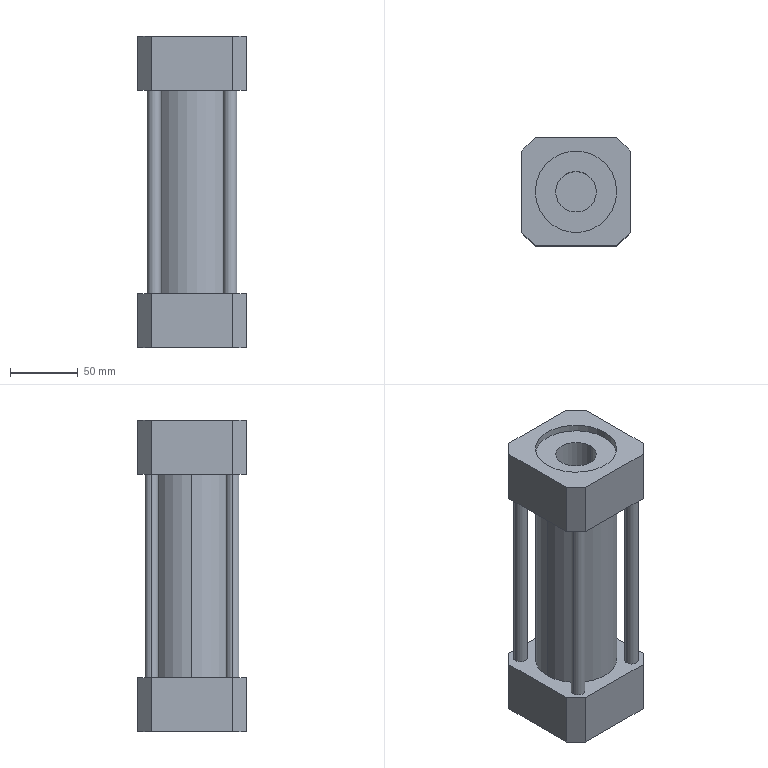Part | STEP file | Chamfer 1-34 | 1 solid | 36 faces | box 80 x 80 x 230 mm | volume 847073 mm3 | plane 22 | cylinder 14 | commonest cylinder face diameters 10 x8 60 x4 30 x2
STEP:
#1=CARTESIAN_POINT('',(-1413.738,1814.264,2528.5));
#2=VERTEX_POINT('',#1);
#3=CARTESIAN_POINT('',(-1383.738,1814.264,2528.5));
#4=VERTEX_POINT('',#3);
#5=CARTESIAN_POINT('',(-1398.738,1814.264,2528.5));
#6=DIRECTION('',(0.,0.,1.));
#7=DIRECTION('',(1.,0.,0.));
#8=AXIS2_PLACEMENT_3D('',#5,#6,#7);
#9=CIRCLE('',#8,15.);
#10=EDGE_CURVE('',#2,#4,#9,.T.);
#11=ORIENTED_EDGE('',*,*,#10,.F.);
#12=CARTESIAN_POINT('',(-1413.738,1814.264,2678.5));
#13=VERTEX_POINT('',#12);
#14=CARTESIAN_POINT('',(-1413.738,1814.264,2528.5));
#15=DIRECTION('',(0.,0.,-1.));
#16=VECTOR('',#15,1000.);
#17=LINE('',#14,#16);
#18=EDGE_CURVE('',#13,#2,#17,.T.);
#19=ORIENTED_EDGE('',*,*,#18,.F.);
#20=CARTESIAN_POINT('',(-1383.738,1814.264,2678.5));
#21=VERTEX_POINT('',#20);
#22=CARTESIAN_POINT('',(-1398.738,1814.264,2678.5));
#23=DIRECTION('',(0.,0.,1.));
#24=DIRECTION('',(1.,0.,0.));
#25=AXIS2_PLACEMENT_3D('',#22,#23,#24);
#26=CIRCLE('',#25,15.);
#27=EDGE_CURVE('',#13,#21,#26,.T.);
#28=ORIENTED_EDGE('',*,*,#27,.T.);
#29=CARTESIAN_POINT('',(-1383.738,1814.264,2528.5));
#30=DIRECTION('',(0.,0.,-1.));
#31=VECTOR('',#30,1000.);
#32=LINE('',#29,#31);
#33=EDGE_CURVE('',#21,#4,#32,.T.);
#34=ORIENTED_EDGE('',*,*,#33,.T.);
#35=EDGE_LOOP('',(#11,#19,#28,#34));
#36=FACE_OUTER_BOUND('',#35,.T.);
#37=CARTESIAN_POINT('',(-1398.738,1814.264,2528.5));
#38=DIRECTION('',(0.,0.,1.));
#39=DIRECTION('',(-1.,0.,0.));
#40=AXIS2_PLACEMENT_3D('',#37,#38,#39);
#41=CYLINDRICAL_SURFACE('',#40,15.);
#42=ADVANCED_FACE('',(#36),#41,.F.);
#43=CARTESIAN_POINT('',(-1428.738,1814.264,2678.5));
#44=VERTEX_POINT('',#43);
#45=CARTESIAN_POINT('',(-1368.738,1814.264,2678.5));
#46=VERTEX_POINT('',#45);
#47=CARTESIAN_POINT('',(-1398.738,1814.264,2678.5));
#48=DIRECTION('',(0.,0.,1.));
#49=DIRECTION('',(1.,0.,0.));
#50=AXIS2_PLACEMENT_3D('',#47,#48,#49);
#51=CIRCLE('',#50,30.);
#52=EDGE_CURVE('',#44,#46,#51,.T.);
#53=ORIENTED_EDGE('',*,*,#52,.F.);
#54=CARTESIAN_POINT('',(-1428.738,1814.264,2683.5));
#55=VERTEX_POINT('',#54);
#56=CARTESIAN_POINT('',(-1428.738,1814.264,2678.5));
#57=DIRECTION('',(0.,0.,-1.));
#58=VECTOR('',#57,1000.);
#59=LINE('',#56,#58);
#60=EDGE_CURVE('',#55,#44,#59,.T.);
#61=ORIENTED_EDGE('',*,*,#60,.F.);
#62=CARTESIAN_POINT('',(-1368.738,1814.264,2683.5));
#63=VERTEX_POINT('',#62);
#64=CARTESIAN_POINT('',(-1398.738,1814.264,2683.5));
#65=DIRECTION('',(0.,0.,1.));
#66=DIRECTION('',(1.,0.,0.));
#67=AXIS2_PLACEMENT_3D('',#64,#65,#66);
#68=CIRCLE('',#67,30.);
#69=EDGE_CURVE('',#55,#63,#68,.T.);
#70=ORIENTED_EDGE('',*,*,#69,.T.);
#71=CARTESIAN_POINT('',(-1368.738,1814.264,2678.5));
#72=DIRECTION('',(0.,0.,-1.));
#73=VECTOR('',#72,1000.);
#74=LINE('',#71,#73);
#75=EDGE_CURVE('',#63,#46,#74,.T.);
#76=ORIENTED_EDGE('',*,*,#75,.T.);
#77=EDGE_LOOP('',(#53,#61,#70,#76));
#78=FACE_OUTER_BOUND('',#77,.T.);
#79=CARTESIAN_POINT('',(-1398.738,1814.264,2678.5));
#80=DIRECTION('',(0.,0.,1.));
#81=DIRECTION('',(-1.,0.,0.));
#82=AXIS2_PLACEMENT_3D('',#79,#80,#81);
#83=CYLINDRICAL_SURFACE('',#82,30.);
#84=ADVANCED_FACE('',(#78),#83,.F.);
#85=CARTESIAN_POINT('',(-1365.738,1844.264,2643.5));
#86=VERTEX_POINT('',#85);
#87=CARTESIAN_POINT('',(-1375.738,1844.264,2643.5));
#88=VERTEX_POINT('',#87);
#89=CARTESIAN_POINT('',(-1370.738,1844.264,2643.5));
#90=DIRECTION('',(0.,0.,1.));
#91=DIRECTION('',(-1.,0.,0.));
#92=AXIS2_PLACEMENT_3D('',#89,#90,#91);
#93=CIRCLE('',#92,5.);
#94=EDGE_CURVE('',#86,#88,#93,.T.);
#95=ORIENTED_EDGE('',*,*,#94,.F.);
#96=CARTESIAN_POINT('',(-1365.738,1844.264,2493.5));
#97=VERTEX_POINT('',#96);
#98=CARTESIAN_POINT('',(-1365.738,1844.264,2643.5));
#99=DIRECTION('',(0.,0.,-1.));
#100=VECTOR('',#99,1000.);
#101=LINE('',#98,#100);
#102=EDGE_CURVE('',#86,#97,#101,.T.);
#103=ORIENTED_EDGE('',*,*,#102,.T.);
#104=CARTESIAN_POINT('',(-1375.738,1844.264,2493.5));
#105=VERTEX_POINT('',#104);
#106=CARTESIAN_POINT('',(-1370.738,1844.264,2493.5));
#107=DIRECTION('',(0.,0.,1.));
#108=DIRECTION('',(-1.,0.,0.));
#109=AXIS2_PLACEMENT_3D('',#106,#107,#108);
#110=CIRCLE('',#109,5.);
#111=EDGE_CURVE('',#97,#105,#110,.T.);
#112=ORIENTED_EDGE('',*,*,#111,.T.);
#113=CARTESIAN_POINT('',(-1375.738,1844.264,2643.5));
#114=DIRECTION('',(0.,0.,-1.));
#115=VECTOR('',#114,1000.);
#116=LINE('',#113,#115);
#117=EDGE_CURVE('',#88,#105,#116,.T.);
#118=ORIENTED_EDGE('',*,*,#117,.F.);
#119=EDGE_LOOP('',(#95,#103,#112,#118));
#120=FACE_OUTER_BOUND('',#119,.T.);
#121=CARTESIAN_POINT('',(-1370.738,1844.264,2643.5));
#122=DIRECTION('',(0.,0.,-1.));
#123=DIRECTION('',(1.,0.,0.));
#124=AXIS2_PLACEMENT_3D('',#121,#122,#123);
#125=CYLINDRICAL_SURFACE('',#124,5.);
#126=ADVANCED_FACE('',(#120),#125,.T.);
#127=CARTESIAN_POINT('',(-1365.738,1784.264,2643.5));
#128=VERTEX_POINT('',#127);
#129=CARTESIAN_POINT('',(-1375.738,1784.264,2643.5));
#130=VERTEX_POINT('',#129);
#131=CARTESIAN_POINT('',(-1370.738,1784.264,2643.5));
#132=DIRECTION('',(0.,0.,1.));
#133=DIRECTION('',(-1.,0.,0.));
#134=AXIS2_PLACEMENT_3D('',#131,#132,#133);
#135=CIRCLE('',#134,5.);
#136=EDGE_CURVE('',#128,#130,#135,.T.);
#137=ORIENTED_EDGE('',*,*,#136,.F.);
#138=CARTESIAN_POINT('',(-1365.738,1784.264,2493.5));
#139=VERTEX_POINT('',#138);
#140=CARTESIAN_POINT('',(-1365.738,1784.264,2643.5));
#141=DIRECTION('',(0.,0.,-1.));
#142=VECTOR('',#141,1000.);
#143=LINE('',#140,#142);
#144=EDGE_CURVE('',#128,#139,#143,.T.);
#145=ORIENTED_EDGE('',*,*,#144,.T.);
#146=CARTESIAN_POINT('',(-1375.738,1784.264,2493.5));
#147=VERTEX_POINT('',#146);
#148=CARTESIAN_POINT('',(-1370.738,1784.264,2493.5));
#149=DIRECTION('',(0.,0.,1.));
#150=DIRECTION('',(-1.,0.,0.));
#151=AXIS2_PLACEMENT_3D('',#148,#149,#150);
#152=CIRCLE('',#151,5.);
#153=EDGE_CURVE('',#139,#147,#152,.T.);
#154=ORIENTED_EDGE('',*,*,#153,.T.);
#155=CARTESIAN_POINT('',(-1375.738,1784.264,2643.5));
#156=DIRECTION('',(0.,0.,-1.));
#157=VECTOR('',#156,1000.);
#158=LINE('',#155,#157);
#159=EDGE_CURVE('',#130,#147,#158,.T.);
#160=ORIENTED_EDGE('',*,*,#159,.F.);
#161=EDGE_LOOP('',(#137,#145,#154,#160));
#162=FACE_OUTER_BOUND('',#161,.T.);
#163=CARTESIAN_POINT('',(-1370.738,1784.264,2643.5));
#164=DIRECTION('',(0.,0.,-1.));
#165=DIRECTION('',(1.,0.,0.));
#166=AXIS2_PLACEMENT_3D('',#163,#164,#165);
#167=CYLINDRICAL_SURFACE('',#166,5.);
#168=ADVANCED_FACE('',(#162),#167,.T.);
#169=CARTESIAN_POINT('',(-1421.738,1784.264,2643.5));
#170=VERTEX_POINT('',#169);
#171=CARTESIAN_POINT('',(-1431.738,1784.264,2643.5));
#172=VERTEX_POINT('',#171);
#173=CARTESIAN_POINT('',(-1426.738,1784.264,2643.5));
#174=DIRECTION('',(0.,0.,1.));
#175=DIRECTION('',(1.,0.,0.));
#176=AXIS2_PLACEMENT_3D('',#173,#174,#175);
#177=CIRCLE('',#176,5.);
#178=EDGE_CURVE('',#170,#172,#177,.T.);
#179=ORIENTED_EDGE('',*,*,#178,.F.);
#180=CARTESIAN_POINT('',(-1421.738,1784.264,2493.5));
#181=VERTEX_POINT('',#180);
#182=CARTESIAN_POINT('',(-1421.738,1784.264,2643.5));
#183=DIRECTION('',(0.,0.,-1.));
#184=VECTOR('',#183,1000.);
#185=LINE('',#182,#184);
#186=EDGE_CURVE('',#170,#181,#185,.T.);
#187=ORIENTED_EDGE('',*,*,#186,.T.);
#188=CARTESIAN_POINT('',(-1431.738,1784.264,2493.5));
#189=VERTEX_POINT('',#188);
#190=CARTESIAN_POINT('',(-1426.738,1784.264,2493.5));
#191=DIRECTION('',(0.,0.,1.));
#192=DIRECTION('',(1.,0.,0.));
#193=AXIS2_PLACEMENT_3D('',#190,#191,#192);
#194=CIRCLE('',#193,5.);
#195=EDGE_CURVE('',#181,#189,#194,.T.);
#196=ORIENTED_EDGE('',*,*,#195,.T.);
#197=CARTESIAN_POINT('',(-1431.738,1784.264,2643.5));
#198=DIRECTION('',(0.,0.,-1.));
#199=VECTOR('',#198,1000.);
#200=LINE('',#197,#199);
#201=EDGE_CURVE('',#172,#189,#200,.T.);
#202=ORIENTED_EDGE('',*,*,#201,.F.);
#203=EDGE_LOOP('',(#179,#187,#196,#202));
#204=FACE_OUTER_BOUND('',#203,.T.);
#205=CARTESIAN_POINT('',(-1426.738,1784.264,2643.5));
#206=DIRECTION('',(0.,0.,-1.));
#207=DIRECTION('',(1.,0.,0.));
#208=AXIS2_PLACEMENT_3D('',#205,#206,#207);
#209=CYLINDRICAL_SURFACE('',#208,5.);
#210=ADVANCED_FACE('',(#204),#209,.T.);
#211=CARTESIAN_POINT('',(-1421.738,1844.264,2643.5));
#212=VERTEX_POINT('',#211);
#213=CARTESIAN_POINT('',(-1431.738,1844.264,2643.5));
#214=VERTEX_POINT('',#213);
#215=CARTESIAN_POINT('',(-1426.738,1844.264,2643.5));
#216=DIRECTION('',(0.,0.,1.));
#217=DIRECTION('',(1.,0.,0.));
#218=AXIS2_PLACEMENT_3D('',#215,#216,#217);
#219=CIRCLE('',#218,5.);
#220=EDGE_CURVE('',#212,#214,#219,.T.);
#221=ORIENTED_EDGE('',*,*,#220,.F.);
#222=CARTESIAN_POINT('',(-1421.738,1844.264,2493.5));
#223=VERTEX_POINT('',#222);
#224=CARTESIAN_POINT('',(-1421.738,1844.264,2643.5));
#225=DIRECTION('',(0.,0.,-1.));
#226=VECTOR('',#225,1000.);
#227=LINE('',#224,#226);
#228=EDGE_CURVE('',#212,#223,#227,.T.);
#229=ORIENTED_EDGE('',*,*,#228,.T.);
#230=CARTESIAN_POINT('',(-1431.738,1844.264,2493.5));
#231=VERTEX_POINT('',#230);
#232=CARTESIAN_POINT('',(-1426.738,1844.264,2493.5));
#233=DIRECTION('',(0.,0.,1.));
#234=DIRECTION('',(1.,0.,0.));
#235=AXIS2_PLACEMENT_3D('',#232,#233,#234);
#236=CIRCLE('',#235,5.);
#237=EDGE_CURVE('',#223,#231,#236,.T.);
#238=ORIENTED_EDGE('',*,*,#237,.T.);
#239=CARTESIAN_POINT('',(-1431.738,1844.264,2643.5));
#240=DIRECTION('',(0.,0.,-1.));
#241=VECTOR('',#240,1000.);
#242=LINE('',#239,#241);
#243=EDGE_CURVE('',#214,#231,#242,.T.);
#244=ORIENTED_EDGE('',*,*,#243,.F.);
#245=EDGE_LOOP('',(#221,#229,#238,#244));
#246=FACE_OUTER_BOUND('',#245,.T.);
#247=CARTESIAN_POINT('',(-1426.738,1844.264,2643.5));
#248=DIRECTION('',(0.,0.,-1.));
#249=DIRECTION('',(1.,0.,0.));
#250=AXIS2_PLACEMENT_3D('',#247,#248,#249);
#251=CYLINDRICAL_SURFACE('',#250,5.);
#252=ADVANCED_FACE('',(#246),#251,.T.);
#253=CARTESIAN_POINT('',(-1368.738,1814.264,2643.5));
#254=VERTEX_POINT('',#253);
#255=CARTESIAN_POINT('',(-1428.738,1814.264,2643.5));
#256=VERTEX_POINT('',#255);
#257=CARTESIAN_POINT('',(-1398.738,1814.264,2643.5));
#258=DIRECTION('',(0.,0.,1.));
#259=DIRECTION('',(1.,0.,0.));
#260=AXIS2_PLACEMENT_3D('',#257,#258,#259);
#261=CIRCLE('',#260,30.);
#262=EDGE_CURVE('',#254,#256,#261,.T.);
#263=ORIENTED_EDGE('',*,*,#262,.F.);
#264=CARTESIAN_POINT('',(-1368.738,1814.264,2493.5));
#265=VERTEX_POINT('',#264);
#266=CARTESIAN_POINT('',(-1368.738,1814.264,2643.5));
#267=DIRECTION('',(0.,0.,-1.));
#268=VECTOR('',#267,1000.);
#269=LINE('',#266,#268);
#270=EDGE_CURVE('',#254,#265,#269,.T.);
#271=ORIENTED_EDGE('',*,*,#270,.T.);
#272=CARTESIAN_POINT('',(-1428.738,1814.264,2493.5));
#273=VERTEX_POINT('',#272);
#274=CARTESIAN_POINT('',(-1398.738,1814.264,2493.5));
#275=DIRECTION('',(0.,0.,1.));
#276=DIRECTION('',(1.,0.,0.));
#277=AXIS2_PLACEMENT_3D('',#274,#275,#276);
#278=CIRCLE('',#277,30.);
#279=EDGE_CURVE('',#265,#273,#278,.T.);
#280=ORIENTED_EDGE('',*,*,#279,.T.);
#281=CARTESIAN_POINT('',(-1428.738,1814.264,2643.5));
#282=DIRECTION('',(0.,0.,-1.));
#283=VECTOR('',#282,1000.);
#284=LINE('',#281,#283);
#285=EDGE_CURVE('',#256,#273,#284,.T.);
#286=ORIENTED_EDGE('',*,*,#285,.F.);
#287=EDGE_LOOP('',(#263,#271,#280,#286));
#288=FACE_OUTER_BOUND('',#287,.T.);
#289=CARTESIAN_POINT('',(-1398.738,1814.264,2643.5));
#290=DIRECTION('',(0.,0.,-1.));
#291=DIRECTION('',(1.,0.,0.));
#292=AXIS2_PLACEMENT_3D('',#289,#290,#291);
#293=CYLINDRICAL_SURFACE('',#292,30.);
#294=ADVANCED_FACE('',(#288),#293,.T.);
#295=CARTESIAN_POINT('',(-1370.738,1784.264,2493.5));
#296=DIRECTION('',(0.,0.,1.));
#297=DIRECTION('',(-1.,0.,0.));
#298=AXIS2_PLACEMENT_3D('',#295,#296,#297);
#299=CIRCLE('',#298,5.);
#300=EDGE_CURVE('',#147,#139,#299,.T.);
#301=ORIENTED_EDGE('',*,*,#300,.F.);
#302=ORIENTED_EDGE('',*,*,#153,.F.);
#303=EDGE_LOOP('',(#301,#302));
#304=FACE_BOUND('',#303,.T.);
#305=CARTESIAN_POINT('',(-1426.738,1844.264,2493.5));
#306=DIRECTION('',(0.,0.,1.));
#307=DIRECTION('',(1.,0.,0.));
#308=AXIS2_PLACEMENT_3D('',#305,#306,#307);
#309=CIRCLE('',#308,5.);
#310=EDGE_CURVE('',#231,#223,#309,.T.);
#311=ORIENTED_EDGE('',*,*,#310,.F.);
#312=ORIENTED_EDGE('',*,*,#237,.F.);
#313=EDGE_LOOP('',(#311,#312));
#314=FACE_BOUND('',#313,.T.);
#315=CARTESIAN_POINT('',(-1438.738,1844.264,2493.5));
#316=VERTEX_POINT('',#315);
#317=CARTESIAN_POINT('',(-1438.738,1784.264,2493.5));
#318=VERTEX_POINT('',#317);
#319=CARTESIAN_POINT('',(-1438.738,1854.264,2493.5));
#320=DIRECTION('',(0.,-1.,0.));
#321=VECTOR('',#320,1000.);
#322=LINE('',#319,#321);
#323=EDGE_CURVE('',#316,#318,#322,.T.);
#324=ORIENTED_EDGE('',*,*,#323,.T.);
#325=CARTESIAN_POINT('',(-1428.738,1774.264,2493.5));
#326=VERTEX_POINT('',#325);
#327=CARTESIAN_POINT('',(-1433.738,1779.264,2493.5));
#328=DIRECTION('',(0.7071,-0.7071,0.));
#329=VECTOR('',#328,1000.);
#330=LINE('',#327,#329);
#331=EDGE_CURVE('',#318,#326,#330,.T.);
#332=ORIENTED_EDGE('',*,*,#331,.T.);
#333=CARTESIAN_POINT('',(-1368.738,1774.264,2493.5));
#334=VERTEX_POINT('',#333);
#335=CARTESIAN_POINT('',(-1438.738,1774.264,2493.5));
#336=DIRECTION('',(1.,0.,0.));
#337=VECTOR('',#336,1000.);
#338=LINE('',#335,#337);
#339=EDGE_CURVE('',#326,#334,#338,.T.);
#340=ORIENTED_EDGE('',*,*,#339,.T.);
#341=CARTESIAN_POINT('',(-1358.738,1784.264,2493.5));
#342=VERTEX_POINT('',#341);
#343=CARTESIAN_POINT('',(-1363.738,1779.264,2493.5));
#344=DIRECTION('',(0.7071,0.7071,0.));
#345=VECTOR('',#344,1000.);
#346=LINE('',#343,#345);
#347=EDGE_CURVE('',#334,#342,#346,.T.);
#348=ORIENTED_EDGE('',*,*,#347,.T.);
#349=CARTESIAN_POINT('',(-1358.738,1844.264,2493.5));
#350=VERTEX_POINT('',#349);
#351=CARTESIAN_POINT('',(-1358.738,1854.264,2493.5));
#352=DIRECTION('',(0.,1.,0.));
#353=VECTOR('',#352,1000.);
#354=LINE('',#351,#353);
#355=EDGE_CURVE('',#342,#350,#354,.T.);
#356=ORIENTED_EDGE('',*,*,#355,.T.);
#357=CARTESIAN_POINT('',(-1368.738,1854.264,2493.5));
#358=VERTEX_POINT('',#357);
#359=CARTESIAN_POINT('',(-1363.738,1849.264,2493.5));
#360=DIRECTION('',(-0.7071,0.7071,0.));
#361=VECTOR('',#360,1000.);
#362=LINE('',#359,#361);
#363=EDGE_CURVE('',#350,#358,#362,.T.);
#364=ORIENTED_EDGE('',*,*,#363,.T.);
#365=CARTESIAN_POINT('',(-1428.738,1854.264,2493.5));
#366=VERTEX_POINT('',#365);
#367=CARTESIAN_POINT('',(-1438.738,1854.264,2493.5));
#368=DIRECTION('',(-1.,0.,0.));
#369=VECTOR('',#368,1000.);
#370=LINE('',#367,#369);
#371=EDGE_CURVE('',#358,#366,#370,.T.);
#372=ORIENTED_EDGE('',*,*,#371,.T.);
#373=CARTESIAN_POINT('',(-1433.738,1849.264,2493.5));
#374=DIRECTION('',(-0.7071,-0.7071,0.));
#375=VECTOR('',#374,1000.);
#376=LINE('',#373,#375);
#377=EDGE_CURVE('',#366,#316,#376,.T.);
#378=ORIENTED_EDGE('',*,*,#377,.T.);
#379=EDGE_LOOP('',(#324,#332,#340,#348,#356,#364,#372,#378));
#380=FACE_OUTER_BOUND('',#379,.T.);
#381=CARTESIAN_POINT('',(-1398.738,1814.264,2493.5));
#382=DIRECTION('',(0.,0.,1.));
#383=DIRECTION('',(1.,0.,0.));
#384=AXIS2_PLACEMENT_3D('',#381,#382,#383);
#385=CIRCLE('',#384,30.);
#386=EDGE_CURVE('',#273,#265,#385,.T.);
#387=ORIENTED_EDGE('',*,*,#386,.F.);
#388=ORIENTED_EDGE('',*,*,#279,.F.);
#389=EDGE_LOOP('',(#387,#388));
#390=FACE_BOUND('',#389,.T.);
#391=CARTESIAN_POINT('',(-1426.738,1784.264,2493.5));
#392=DIRECTION('',(0.,0.,1.));
#393=DIRECTION('',(1.,0.,0.));
#394=AXIS2_PLACEMENT_3D('',#391,#392,#393);
#395=CIRCLE('',#394,5.);
#396=EDGE_CURVE('',#189,#181,#395,.T.);
#397=ORIENTED_EDGE('',*,*,#396,.F.);
#398=ORIENTED_EDGE('',*,*,#195,.F.);
#399=EDGE_LOOP('',(#397,#398));
#400=FACE_BOUND('',#399,.T.);
#401=CARTESIAN_POINT('',(-1370.738,1844.264,2493.5));
#402=DIRECTION('',(0.,0.,1.));
#403=DIRECTION('',(-1.,0.,0.));
#404=AXIS2_PLACEMENT_3D('',#401,#402,#403);
#405=CIRCLE('',#404,5.);
#406=EDGE_CURVE('',#105,#97,#405,.T.);
#407=ORIENTED_EDGE('',*,*,#406,.F.);
#408=ORIENTED_EDGE('',*,*,#111,.F.);
#409=EDGE_LOOP('',(#407,#408));
#410=FACE_BOUND('',#409,.T.);
#411=CARTESIAN_POINT('',(-1398.738,1814.264,2493.5));
#412=DIRECTION('',(0.,0.,1.));
#413=DIRECTION('',(-1.,0.,0.));
#414=AXIS2_PLACEMENT_3D('',#411,#412,#413);
#415=PLANE('',#414);
#416=ADVANCED_FACE('',(#304,#314,#380,#390,#400,#410),#415,.T.);
#417=ORIENTED_EDGE('',*,*,#355,.F.);
#418=CARTESIAN_POINT('',(-1358.738,1784.264,2453.5));
#419=VERTEX_POINT('',#418);
#420=CARTESIAN_POINT('',(-1358.738,1784.264,2493.5));
#421=DIRECTION('',(0.,0.,-1.));
#422=VECTOR('',#421,1000.);
#423=LINE('',#420,#422);
#424=EDGE_CURVE('',#342,#419,#423,.T.);
#425=ORIENTED_EDGE('',*,*,#424,.T.);
#426=CARTESIAN_POINT('',(-1358.738,1844.264,2453.5));
#427=VERTEX_POINT('',#426);
#428=CARTESIAN_POINT('',(-1358.738,1854.264,2453.5));
#429=DIRECTION('',(0.,1.,0.));
#430=VECTOR('',#429,1000.);
#431=LINE('',#428,#430);
#432=EDGE_CURVE('',#419,#427,#431,.T.);
#433=ORIENTED_EDGE('',*,*,#432,.T.);
#434=CARTESIAN_POINT('',(-1358.738,1844.264,2493.5));
#435=DIRECTION('',(0.,0.,1.));
#436=VECTOR('',#435,1000.);
#437=LINE('',#434,#436);
#438=EDGE_CURVE('',#427,#350,#437,.T.);
#439=ORIENTED_EDGE('',*,*,#438,.T.);
#440=EDGE_LOOP('',(#417,#425,#433,#439));
#441=FACE_OUTER_BOUND('',#440,.T.);
#442=CARTESIAN_POINT('',(-1358.738,1854.264,2493.5));
#443=DIRECTION('',(-1.,0.,0.));
#444=DIRECTION('',(0.,1.,0.));
#445=AXIS2_PLACEMENT_3D('',#442,#443,#444);
#446=PLANE('',#445);
#447=ADVANCED_FACE('',(#441),#446,.F.);
#448=ORIENTED_EDGE('',*,*,#371,.F.);
#449=CARTESIAN_POINT('',(-1368.738,1854.264,2453.5));
#450=VERTEX_POINT('',#449);
#451=CARTESIAN_POINT('',(-1368.738,1854.264,2493.5));
#452=DIRECTION('',(0.,0.,-1.));
#453=VECTOR('',#452,1000.);
#454=LINE('',#451,#453);
#455=EDGE_CURVE('',#358,#450,#454,.T.);
#456=ORIENTED_EDGE('',*,*,#455,.T.);
#457=CARTESIAN_POINT('',(-1428.738,1854.264,2453.5));
#458=VERTEX_POINT('',#457);
#459=CARTESIAN_POINT('',(-1438.738,1854.264,2453.5));
#460=DIRECTION('',(-1.,0.,0.));
#461=VECTOR('',#460,1000.);
#462=LINE('',#459,#461);
#463=EDGE_CURVE('',#450,#458,#462,.T.);
#464=ORIENTED_EDGE('',*,*,#463,.T.);
#465=CARTESIAN_POINT('',(-1428.738,1854.264,2493.5));
#466=DIRECTION('',(0.,0.,1.));
#467=VECTOR('',#466,1000.);
#468=LINE('',#465,#467);
#469=EDGE_CURVE('',#458,#366,#468,.T.);
#470=ORIENTED_EDGE('',*,*,#469,.T.);
#471=EDGE_LOOP('',(#448,#456,#464,#470));
#472=FACE_OUTER_BOUND('',#471,.T.);
#473=CARTESIAN_POINT('',(-1438.738,1854.264,2493.5));
#474=DIRECTION('',(0.,-1.,0.));
#475=DIRECTION('',(-1.,0.,0.));
#476=AXIS2_PLACEMENT_3D('',#473,#474,#475);
#477=PLANE('',#476);
#478=ADVANCED_FACE('',(#472),#477,.F.);
#479=CARTESIAN_POINT('',(-1438.738,1844.264,2453.5));
#480=VERTEX_POINT('',#479);
#481=CARTESIAN_POINT('',(-1438.738,1784.264,2453.5));
#482=VERTEX_POINT('',#481);
#483=CARTESIAN_POINT('',(-1438.738,1854.264,2453.5));
#484=DIRECTION('',(0.,-1.,0.));
#485=VECTOR('',#484,1000.);
#486=LINE('',#483,#485);
#487=EDGE_CURVE('',#480,#482,#486,.T.);
#488=ORIENTED_EDGE('',*,*,#487,.T.);
#489=CARTESIAN_POINT('',(-1438.738,1784.264,2493.5));
#490=DIRECTION('',(0.,0.,1.));
#491=VECTOR('',#490,1000.);
#492=LINE('',#489,#491);
#493=EDGE_CURVE('',#482,#318,#492,.T.);
#494=ORIENTED_EDGE('',*,*,#493,.T.);
#495=ORIENTED_EDGE('',*,*,#323,.F.);
#496=CARTESIAN_POINT('',(-1438.738,1844.264,2493.5));
#497=DIRECTION('',(0.,0.,-1.));
#498=VECTOR('',#497,1000.);
#499=LINE('',#496,#498);
#500=EDGE_CURVE('',#316,#480,#499,.T.);
#501=ORIENTED_EDGE('',*,*,#500,.T.);
#502=EDGE_LOOP('',(#488,#494,#495,#501));
#503=FACE_OUTER_BOUND('',#502,.T.);
#504=CARTESIAN_POINT('',(-1438.738,1854.264,2493.5));
#505=DIRECTION('',(1.,0.,0.));
#506=DIRECTION('',(0.,-1.,0.));
#507=AXIS2_PLACEMENT_3D('',#504,#505,#506);
#508=PLANE('',#507);
#509=ADVANCED_FACE('',(#503),#508,.F.);
#510=ORIENTED_EDGE('',*,*,#339,.F.);
#511=CARTESIAN_POINT('',(-1428.738,1774.264,2453.5));
#512=VERTEX_POINT('',#511);
#513=CARTESIAN_POINT('',(-1428.738,1774.264,2493.5));
#514=DIRECTION('',(0.,0.,-1.));
#515=VECTOR('',#514,1000.);
#516=LINE('',#513,#515);
#517=EDGE_CURVE('',#326,#512,#516,.T.);
#518=ORIENTED_EDGE('',*,*,#517,.T.);
#519=CARTESIAN_POINT('',(-1368.738,1774.264,2453.5));
#520=VERTEX_POINT('',#519);
#521=CARTESIAN_POINT('',(-1438.738,1774.264,2453.5));
#522=DIRECTION('',(1.,0.,0.));
#523=VECTOR('',#522,1000.);
#524=LINE('',#521,#523);
#525=EDGE_CURVE('',#512,#520,#524,.T.);
#526=ORIENTED_EDGE('',*,*,#525,.T.);
#527=CARTESIAN_POINT('',(-1368.738,1774.264,2493.5));
#528=DIRECTION('',(0.,0.,1.));
#529=VECTOR('',#528,1000.);
#530=LINE('',#527,#529);
#531=EDGE_CURVE('',#520,#334,#530,.T.);
#532=ORIENTED_EDGE('',*,*,#531,.T.);
#533=EDGE_LOOP('',(#510,#518,#526,#532));
#534=FACE_OUTER_BOUND('',#533,.T.);
#535=CARTESIAN_POINT('',(-1438.738,1774.264,2493.5));
#536=DIRECTION('',(0.,1.,0.));
#537=DIRECTION('',(1.,0.,0.));
#538=AXIS2_PLACEMENT_3D('',#535,#536,#537);
#539=PLANE('',#538);
#540=ADVANCED_FACE('',(#534),#539,.F.);
#541=ORIENTED_EDGE('',*,*,#525,.F.);
#542=CARTESIAN_POINT('',(-1428.738,1774.264,2453.5));
#543=DIRECTION('',(-0.7071,0.7071,0.));
#544=VECTOR('',#543,1000.);
#545=LINE('',#542,#544);
#546=EDGE_CURVE('',#512,#482,#545,.T.);
#547=ORIENTED_EDGE('',*,*,#546,.T.);
#548=ORIENTED_EDGE('',*,*,#487,.F.);
#549=CARTESIAN_POINT('',(-1438.738,1844.264,2453.5));
#550=DIRECTION('',(0.7071,0.7071,0.));
#551=VECTOR('',#550,1000.);
#552=LINE('',#549,#551);
#553=EDGE_CURVE('',#480,#458,#552,.T.);
#554=ORIENTED_EDGE('',*,*,#553,.T.);
#555=ORIENTED_EDGE('',*,*,#463,.F.);
#556=CARTESIAN_POINT('',(-1368.738,1854.264,2453.5));
#557=DIRECTION('',(0.7071,-0.7071,0.));
#558=VECTOR('',#557,1000.);
#559=LINE('',#556,#558);
#560=EDGE_CURVE('',#450,#427,#559,.T.);
#561=ORIENTED_EDGE('',*,*,#560,.T.);
#562=ORIENTED_EDGE('',*,*,#432,.F.);
#563=CARTESIAN_POINT('',(-1358.738,1784.264,2453.5));
#564=DIRECTION('',(-0.7071,-0.7071,0.));
#565=VECTOR('',#564,1000.);
#566=LINE('',#563,#565);
#567=EDGE_CURVE('',#419,#520,#566,.T.);
#568=ORIENTED_EDGE('',*,*,#567,.T.);
#569=EDGE_LOOP('',(#541,#547,#548,#554,#555,#561,#562,#568));
#570=FACE_OUTER_BOUND('',#569,.T.);
#571=CARTESIAN_POINT('',(-1398.738,1814.264,2453.5));
#572=DIRECTION('',(0.,0.,1.));
#573=DIRECTION('',(-1.,0.,0.));
#574=AXIS2_PLACEMENT_3D('',#571,#572,#573);
#575=PLANE('',#574);
#576=ADVANCED_FACE('',(#570),#575,.F.);
#577=ORIENTED_EDGE('',*,*,#270,.F.);
#578=CARTESIAN_POINT('',(-1398.738,1814.264,2643.5));
#579=DIRECTION('',(0.,0.,1.));
#580=DIRECTION('',(1.,0.,0.));
#581=AXIS2_PLACEMENT_3D('',#578,#579,#580);
#582=CIRCLE('',#581,30.);
#583=EDGE_CURVE('',#256,#254,#582,.T.);
#584=ORIENTED_EDGE('',*,*,#583,.F.);
#585=ORIENTED_EDGE('',*,*,#285,.T.);
#586=ORIENTED_EDGE('',*,*,#386,.T.);
#587=EDGE_LOOP('',(#577,#584,#585,#586));
#588=FACE_OUTER_BOUND('',#587,.T.);
#589=CARTESIAN_POINT('',(-1398.738,1814.264,2643.5));
#590=DIRECTION('',(0.,0.,-1.));
#591=DIRECTION('',(1.,0.,0.));
#592=AXIS2_PLACEMENT_3D('',#589,#590,#591);
#593=CYLINDRICAL_SURFACE('',#592,30.);
#594=ADVANCED_FACE('',(#588),#593,.T.);
#595=ORIENTED_EDGE('',*,*,#228,.F.);
#596=CARTESIAN_POINT('',(-1426.738,1844.264,2643.5));
#597=DIRECTION('',(0.,0.,1.));
#598=DIRECTION('',(1.,0.,0.));
#599=AXIS2_PLACEMENT_3D('',#596,#597,#598);
#600=CIRCLE('',#599,5.);
#601=EDGE_CURVE('',#214,#212,#600,.T.);
#602=ORIENTED_EDGE('',*,*,#601,.F.);
#603=ORIENTED_EDGE('',*,*,#243,.T.);
#604=ORIENTED_EDGE('',*,*,#310,.T.);
#605=EDGE_LOOP('',(#595,#602,#603,#604));
#606=FACE_OUTER_BOUND('',#605,.T.);
#607=CARTESIAN_POINT('',(-1426.738,1844.264,2643.5));
#608=DIRECTION('',(0.,0.,-1.));
#609=DIRECTION('',(1.,0.,0.));
#610=AXIS2_PLACEMENT_3D('',#607,#608,#609);
#611=CYLINDRICAL_SURFACE('',#610,5.);
#612=ADVANCED_FACE('',(#606),#611,.T.);
#613=ORIENTED_EDGE('',*,*,#186,.F.);
#614=CARTESIAN_POINT('',(-1426.738,1784.264,2643.5));
#615=DIRECTION('',(0.,0.,1.));
#616=DIRECTION('',(1.,0.,0.));
#617=AXIS2_PLACEMENT_3D('',#614,#615,#616);
#618=CIRCLE('',#617,5.);
#619=EDGE_CURVE('',#172,#170,#618,.T.);
#620=ORIENTED_EDGE('',*,*,#619,.F.);
#621=ORIENTED_EDGE('',*,*,#201,.T.);
#622=ORIENTED_EDGE('',*,*,#396,.T.);
#623=EDGE_LOOP('',(#613,#620,#621,#622));
#624=FACE_OUTER_BOUND('',#623,.T.);
#625=CARTESIAN_POINT('',(-1426.738,1784.264,2643.5));
#626=DIRECTION('',(0.,0.,-1.));
#627=DIRECTION('',(1.,0.,0.));
#628=AXIS2_PLACEMENT_3D('',#625,#626,#627);
#629=CYLINDRICAL_SURFACE('',#628,5.);
#630=ADVANCED_FACE('',(#624),#629,.T.);
#631=ORIENTED_EDGE('',*,*,#144,.F.);
#632=CARTESIAN_POINT('',(-1370.738,1784.264,2643.5));
#633=DIRECTION('',(0.,0.,1.));
#634=DIRECTION('',(-1.,0.,0.));
#635=AXIS2_PLACEMENT_3D('',#632,#633,#634);
#636=CIRCLE('',#635,5.);
#637=EDGE_CURVE('',#130,#128,#636,.T.);
#638=ORIENTED_EDGE('',*,*,#637,.F.);
#639=ORIENTED_EDGE('',*,*,#159,.T.);
#640=ORIENTED_EDGE('',*,*,#300,.T.);
#641=EDGE_LOOP('',(#631,#638,#639,#640));
#642=FACE_OUTER_BOUND('',#641,.T.);
#643=CARTESIAN_POINT('',(-1370.738,1784.264,2643.5));
#644=DIRECTION('',(0.,0.,-1.));
#645=DIRECTION('',(1.,0.,0.));
#646=AXIS2_PLACEMENT_3D('',#643,#644,#645);
#647=CYLINDRICAL_SURFACE('',#646,5.);
#648=ADVANCED_FACE('',(#642),#647,.T.);
#649=ORIENTED_EDGE('',*,*,#102,.F.);
#650=CARTESIAN_POINT('',(-1370.738,1844.264,2643.5));
#651=DIRECTION('',(0.,0.,1.));
#652=DIRECTION('',(-1.,0.,0.));
#653=AXIS2_PLACEMENT_3D('',#650,#651,#652);
#654=CIRCLE('',#653,5.);
#655=EDGE_CURVE('',#88,#86,#654,.T.);
#656=ORIENTED_EDGE('',*,*,#655,.F.);
#657=ORIENTED_EDGE('',*,*,#117,.T.);
#658=ORIENTED_EDGE('',*,*,#406,.T.);
#659=EDGE_LOOP('',(#649,#656,#657,#658));
#660=FACE_OUTER_BOUND('',#659,.T.);
#661=CARTESIAN_POINT('',(-1370.738,1844.264,2643.5));
#662=DIRECTION('',(0.,0.,-1.));
#663=DIRECTION('',(1.,0.,0.));
#664=AXIS2_PLACEMENT_3D('',#661,#662,#663);
#665=CYLINDRICAL_SURFACE('',#664,5.);
#666=ADVANCED_FACE('',(#660),#665,.T.);
#667=ORIENTED_EDGE('',*,*,#601,.T.);
#668=ORIENTED_EDGE('',*,*,#220,.T.);
#669=EDGE_LOOP('',(#667,#668));
#670=FACE_BOUND('',#669,.T.);
#671=ORIENTED_EDGE('',*,*,#637,.T.);
#672=ORIENTED_EDGE('',*,*,#136,.T.);
#673=EDGE_LOOP('',(#671,#672));
#674=FACE_BOUND('',#673,.T.);
#675=CARTESIAN_POINT('',(-1438.738,1844.264,2643.5));
#676=VERTEX_POINT('',#675);
#677=CARTESIAN_POINT('',(-1438.738,1784.264,2643.5));
#678=VERTEX_POINT('',#677);
#679=CARTESIAN_POINT('',(-1438.738,1774.264,2643.5));
#680=DIRECTION('',(0.,-1.,0.));
#681=VECTOR('',#680,1000.);
#682=LINE('',#679,#681);
#683=EDGE_CURVE('',#676,#678,#682,.T.);
#684=ORIENTED_EDGE('',*,*,#683,.F.);
#685=CARTESIAN_POINT('',(-1428.738,1854.264,2643.5));
#686=VERTEX_POINT('',#685);
#687=CARTESIAN_POINT('',(-1433.738,1849.264,2643.5));
#688=DIRECTION('',(0.7071,0.7071,0.));
#689=VECTOR('',#688,1000.);
#690=LINE('',#687,#689);
#691=EDGE_CURVE('',#676,#686,#690,.T.);
#692=ORIENTED_EDGE('',*,*,#691,.T.);
#693=CARTESIAN_POINT('',(-1368.738,1854.264,2643.5));
#694=VERTEX_POINT('',#693);
#695=CARTESIAN_POINT('',(-1438.738,1854.264,2643.5));
#696=DIRECTION('',(-1.,0.,0.));
#697=VECTOR('',#696,1000.);
#698=LINE('',#695,#697);
#699=EDGE_CURVE('',#694,#686,#698,.T.);
#700=ORIENTED_EDGE('',*,*,#699,.F.);
#701=CARTESIAN_POINT('',(-1358.738,1844.264,2643.5));
#702=VERTEX_POINT('',#701);
#703=CARTESIAN_POINT('',(-1363.738,1849.264,2643.5));
#704=DIRECTION('',(0.7071,-0.7071,0.));
#705=VECTOR('',#704,1000.);
#706=LINE('',#703,#705);
#707=EDGE_CURVE('',#694,#702,#706,.T.);
#708=ORIENTED_EDGE('',*,*,#707,.T.);
#709=CARTESIAN_POINT('',(-1358.738,1784.264,2643.5));
#710=VERTEX_POINT('',#709);
#711=CARTESIAN_POINT('',(-1358.738,1774.264,2643.5));
#712=DIRECTION('',(0.,1.,0.));
#713=VECTOR('',#712,1000.);
#714=LINE('',#711,#713);
#715=EDGE_CURVE('',#710,#702,#714,.T.);
#716=ORIENTED_EDGE('',*,*,#715,.F.);
#717=CARTESIAN_POINT('',(-1368.738,1774.264,2643.5));
#718=VERTEX_POINT('',#717);
#719=CARTESIAN_POINT('',(-1363.738,1779.264,2643.5));
#720=DIRECTION('',(-0.7071,-0.7071,0.));
#721=VECTOR('',#720,1000.);
#722=LINE('',#719,#721);
#723=EDGE_CURVE('',#710,#718,#722,.T.);
#724=ORIENTED_EDGE('',*,*,#723,.T.);
#725=CARTESIAN_POINT('',(-1428.738,1774.264,2643.5));
#726=VERTEX_POINT('',#725);
#727=CARTESIAN_POINT('',(-1438.738,1774.264,2643.5));
#728=DIRECTION('',(1.,0.,0.));
#729=VECTOR('',#728,1000.);
#730=LINE('',#727,#729);
#731=EDGE_CURVE('',#726,#718,#730,.T.);
#732=ORIENTED_EDGE('',*,*,#731,.F.);
#733=CARTESIAN_POINT('',(-1433.738,1779.264,2643.5));
#734=DIRECTION('',(-0.7071,0.7071,0.));
#735=VECTOR('',#734,1000.);
#736=LINE('',#733,#735);
#737=EDGE_CURVE('',#726,#678,#736,.T.);
#738=ORIENTED_EDGE('',*,*,#737,.T.);
#739=EDGE_LOOP('',(#684,#692,#700,#708,#716,#724,#732,#738));
#740=FACE_OUTER_BOUND('',#739,.T.);
#741=ORIENTED_EDGE('',*,*,#655,.T.);
#742=ORIENTED_EDGE('',*,*,#94,.T.);
#743=EDGE_LOOP('',(#741,#742));
#744=FACE_BOUND('',#743,.T.);
#745=ORIENTED_EDGE('',*,*,#619,.T.);
#746=ORIENTED_EDGE('',*,*,#178,.T.);
#747=EDGE_LOOP('',(#745,#746));
#748=FACE_BOUND('',#747,.T.);
#749=ORIENTED_EDGE('',*,*,#583,.T.);
#750=ORIENTED_EDGE('',*,*,#262,.T.);
#751=EDGE_LOOP('',(#749,#750));
#752=FACE_BOUND('',#751,.T.);
#753=CARTESIAN_POINT('',(-1398.738,1814.264,2643.5));
#754=DIRECTION('',(0.,0.,-1.));
#755=DIRECTION('',(1.,0.,0.));
#756=AXIS2_PLACEMENT_3D('',#753,#754,#755);
#757=PLANE('',#756);
#758=ADVANCED_FACE('',(#670,#674,#740,#744,#748,#752),#757,.T.);
#759=ORIENTED_EDGE('',*,*,#715,.T.);
#760=CARTESIAN_POINT('',(-1358.738,1844.264,2683.5));
#761=VERTEX_POINT('',#760);
#762=CARTESIAN_POINT('',(-1358.738,1844.264,2683.5));
#763=DIRECTION('',(0.,0.,1.));
#764=VECTOR('',#763,1000.);
#765=LINE('',#762,#764);
#766=EDGE_CURVE('',#702,#761,#765,.T.);
#767=ORIENTED_EDGE('',*,*,#766,.T.);
#768=CARTESIAN_POINT('',(-1358.738,1784.264,2683.5));
#769=VERTEX_POINT('',#768);
#770=CARTESIAN_POINT('',(-1358.738,1774.264,2683.5));
#771=DIRECTION('',(0.,1.,0.));
#772=VECTOR('',#771,1000.);
#773=LINE('',#770,#772);
#774=EDGE_CURVE('',#769,#761,#773,.T.);
#775=ORIENTED_EDGE('',*,*,#774,.F.);
#776=CARTESIAN_POINT('',(-1358.738,1784.264,2683.5));
#777=DIRECTION('',(0.,0.,-1.));
#778=VECTOR('',#777,1000.);
#779=LINE('',#776,#778);
#780=EDGE_CURVE('',#769,#710,#779,.T.);
#781=ORIENTED_EDGE('',*,*,#780,.T.);
#782=EDGE_LOOP('',(#759,#767,#775,#781));
#783=FACE_OUTER_BOUND('',#782,.T.);
#784=CARTESIAN_POINT('',(-1358.738,1774.264,2683.5));
#785=DIRECTION('',(-1.,0.,0.));
#786=DIRECTION('',(0.,0.,-1.));
#787=AXIS2_PLACEMENT_3D('',#784,#785,#786);
#788=PLANE('',#787);
#789=ADVANCED_FACE('',(#783),#788,.F.);
#790=ORIENTED_EDGE('',*,*,#699,.T.);
#791=CARTESIAN_POINT('',(-1428.738,1854.264,2683.5));
#792=VERTEX_POINT('',#791);
#793=CARTESIAN_POINT('',(-1428.738,1854.264,2683.5));
#794=DIRECTION('',(0.,0.,1.));
#795=VECTOR('',#794,1000.);
#796=LINE('',#793,#795);
#797=EDGE_CURVE('',#686,#792,#796,.T.);
#798=ORIENTED_EDGE('',*,*,#797,.T.);
#799=CARTESIAN_POINT('',(-1368.738,1854.264,2683.5));
#800=VERTEX_POINT('',#799);
#801=CARTESIAN_POINT('',(-1438.738,1854.264,2683.5));
#802=DIRECTION('',(-1.,0.,0.));
#803=VECTOR('',#802,1000.);
#804=LINE('',#801,#803);
#805=EDGE_CURVE('',#800,#792,#804,.T.);
#806=ORIENTED_EDGE('',*,*,#805,.F.);
#807=CARTESIAN_POINT('',(-1368.738,1854.264,2683.5));
#808=DIRECTION('',(0.,0.,-1.));
#809=VECTOR('',#808,1000.);
#810=LINE('',#807,#809);
#811=EDGE_CURVE('',#800,#694,#810,.T.);
#812=ORIENTED_EDGE('',*,*,#811,.T.);
#813=EDGE_LOOP('',(#790,#798,#806,#812));
#814=FACE_OUTER_BOUND('',#813,.T.);
#815=CARTESIAN_POINT('',(-1438.738,1854.264,2683.5));
#816=DIRECTION('',(0.,-1.,0.));
#817=DIRECTION('',(-1.,0.,0.));
#818=AXIS2_PLACEMENT_3D('',#815,#816,#817);
#819=PLANE('',#818);
#820=ADVANCED_FACE('',(#814),#819,.F.);
#821=CARTESIAN_POINT('',(-1438.738,1844.264,2683.5));
#822=VERTEX_POINT('',#821);
#823=CARTESIAN_POINT('',(-1438.738,1784.264,2683.5));
#824=VERTEX_POINT('',#823);
#825=CARTESIAN_POINT('',(-1438.738,1774.264,2683.5));
#826=DIRECTION('',(0.,-1.,0.));
#827=VECTOR('',#826,1000.);
#828=LINE('',#825,#827);
#829=EDGE_CURVE('',#822,#824,#828,.T.);
#830=ORIENTED_EDGE('',*,*,#829,.F.);
#831=CARTESIAN_POINT('',(-1438.738,1844.264,2683.5));
#832=DIRECTION('',(0.,0.,-1.));
#833=VECTOR('',#832,1000.);
#834=LINE('',#831,#833);
#835=EDGE_CURVE('',#822,#676,#834,.T.);
#836=ORIENTED_EDGE('',*,*,#835,.T.);
#837=ORIENTED_EDGE('',*,*,#683,.T.);
#838=CARTESIAN_POINT('',(-1438.738,1784.264,2683.5));
#839=DIRECTION('',(0.,0.,1.));
#840=VECTOR('',#839,1000.);
#841=LINE('',#838,#840);
#842=EDGE_CURVE('',#678,#824,#841,.T.);
#843=ORIENTED_EDGE('',*,*,#842,.T.);
#844=EDGE_LOOP('',(#830,#836,#837,#843));
#845=FACE_OUTER_BOUND('',#844,.T.);
#846=CARTESIAN_POINT('',(-1438.738,1774.264,2683.5));
#847=DIRECTION('',(1.,0.,0.));
#848=DIRECTION('',(0.,0.,1.));
#849=AXIS2_PLACEMENT_3D('',#846,#847,#848);
#850=PLANE('',#849);
#851=ADVANCED_FACE('',(#845),#850,.F.);
#852=ORIENTED_EDGE('',*,*,#731,.T.);
#853=CARTESIAN_POINT('',(-1368.738,1774.264,2683.5));
#854=VERTEX_POINT('',#853);
#855=CARTESIAN_POINT('',(-1368.738,1774.264,2683.5));
#856=DIRECTION('',(0.,0.,1.));
#857=VECTOR('',#856,1000.);
#858=LINE('',#855,#857);
#859=EDGE_CURVE('',#718,#854,#858,.T.);
#860=ORIENTED_EDGE('',*,*,#859,.T.);
#861=CARTESIAN_POINT('',(-1428.738,1774.264,2683.5));
#862=VERTEX_POINT('',#861);
#863=CARTESIAN_POINT('',(-1438.738,1774.264,2683.5));
#864=DIRECTION('',(1.,0.,0.));
#865=VECTOR('',#864,1000.);
#866=LINE('',#863,#865);
#867=EDGE_CURVE('',#862,#854,#866,.T.);
#868=ORIENTED_EDGE('',*,*,#867,.F.);
#869=CARTESIAN_POINT('',(-1428.738,1774.264,2683.5));
#870=DIRECTION('',(0.,0.,-1.));
#871=VECTOR('',#870,1000.);
#872=LINE('',#869,#871);
#873=EDGE_CURVE('',#862,#726,#872,.T.);
#874=ORIENTED_EDGE('',*,*,#873,.T.);
#875=EDGE_LOOP('',(#852,#860,#868,#874));
#876=FACE_OUTER_BOUND('',#875,.T.);
#877=CARTESIAN_POINT('',(-1438.738,1774.264,2683.5));
#878=DIRECTION('',(0.,1.,0.));
#879=DIRECTION('',(1.,0.,0.));
#880=AXIS2_PLACEMENT_3D('',#877,#878,#879);
#881=PLANE('',#880);
#882=ADVANCED_FACE('',(#876),#881,.F.);
#883=CARTESIAN_POINT('',(-1398.738,1814.264,2683.5));
#884=DIRECTION('',(0.,0.,1.));
#885=DIRECTION('',(1.,0.,0.));
#886=AXIS2_PLACEMENT_3D('',#883,#884,#885);
#887=CIRCLE('',#886,30.);
#888=EDGE_CURVE('',#63,#55,#887,.T.);
#889=ORIENTED_EDGE('',*,*,#888,.F.);
#890=ORIENTED_EDGE('',*,*,#69,.F.);
#891=EDGE_LOOP('',(#889,#890));
#892=FACE_BOUND('',#891,.T.);
#893=ORIENTED_EDGE('',*,*,#805,.T.);
#894=CARTESIAN_POINT('',(-1438.738,1844.264,2683.5));
#895=DIRECTION('',(-0.7071,-0.7071,0.));
#896=VECTOR('',#895,1000.);
#897=LINE('',#894,#896);
#898=EDGE_CURVE('',#792,#822,#897,.T.);
#899=ORIENTED_EDGE('',*,*,#898,.T.);
#900=ORIENTED_EDGE('',*,*,#829,.T.);
#901=CARTESIAN_POINT('',(-1428.738,1774.264,2683.5));
#902=DIRECTION('',(0.7071,-0.7071,0.));
#903=VECTOR('',#902,1000.);
#904=LINE('',#901,#903);
#905=EDGE_CURVE('',#824,#862,#904,.T.);
#906=ORIENTED_EDGE('',*,*,#905,.T.);
#907=ORIENTED_EDGE('',*,*,#867,.T.);
#908=CARTESIAN_POINT('',(-1358.738,1784.264,2683.5));
#909=DIRECTION('',(0.7071,0.7071,0.));
#910=VECTOR('',#909,1000.);
#911=LINE('',#908,#910);
#912=EDGE_CURVE('',#854,#769,#911,.T.);
#913=ORIENTED_EDGE('',*,*,#912,.T.);
#914=ORIENTED_EDGE('',*,*,#774,.T.);
#915=CARTESIAN_POINT('',(-1368.738,1854.264,2683.5));
#916=DIRECTION('',(-0.7071,0.7071,0.));
#917=VECTOR('',#916,1000.);
#918=LINE('',#915,#917);
#919=EDGE_CURVE('',#761,#800,#918,.T.);
#920=ORIENTED_EDGE('',*,*,#919,.T.);
#921=EDGE_LOOP('',(#893,#899,#900,#906,#907,#913,#914,#920));
#922=FACE_OUTER_BOUND('',#921,.T.);
#923=CARTESIAN_POINT('',(-1398.738,1814.264,2683.5));
#924=DIRECTION('',(0.,0.,-1.));
#925=DIRECTION('',(1.,0.,0.));
#926=AXIS2_PLACEMENT_3D('',#923,#924,#925);
#927=PLANE('',#926);
#928=ADVANCED_FACE('',(#892,#922),#927,.F.);
#929=ORIENTED_EDGE('',*,*,#60,.T.);
#930=CARTESIAN_POINT('',(-1398.738,1814.264,2678.5));
#931=DIRECTION('',(0.,0.,1.));
#932=DIRECTION('',(1.,0.,0.));
#933=AXIS2_PLACEMENT_3D('',#930,#931,#932);
#934=CIRCLE('',#933,30.);
#935=EDGE_CURVE('',#46,#44,#934,.T.);
#936=ORIENTED_EDGE('',*,*,#935,.F.);
#937=ORIENTED_EDGE('',*,*,#75,.F.);
#938=ORIENTED_EDGE('',*,*,#888,.T.);
#939=EDGE_LOOP('',(#929,#936,#937,#938));
#940=FACE_OUTER_BOUND('',#939,.T.);
#941=CARTESIAN_POINT('',(-1398.738,1814.264,2678.5));
#942=DIRECTION('',(0.,0.,1.));
#943=DIRECTION('',(-1.,0.,0.));
#944=AXIS2_PLACEMENT_3D('',#941,#942,#943);
#945=CYLINDRICAL_SURFACE('',#944,30.);
#946=ADVANCED_FACE('',(#940),#945,.F.);
#947=CARTESIAN_POINT('',(-1398.738,1814.264,2678.5));
#948=DIRECTION('',(0.,0.,1.));
#949=DIRECTION('',(1.,0.,0.));
#950=AXIS2_PLACEMENT_3D('',#947,#948,#949);
#951=CIRCLE('',#950,15.);
#952=EDGE_CURVE('',#21,#13,#951,.T.);
#953=ORIENTED_EDGE('',*,*,#952,.F.);
#954=ORIENTED_EDGE('',*,*,#27,.F.);
#955=EDGE_LOOP('',(#953,#954));
#956=FACE_BOUND('',#955,.T.);
#957=ORIENTED_EDGE('',*,*,#935,.T.);
#958=ORIENTED_EDGE('',*,*,#52,.T.);
#959=EDGE_LOOP('',(#957,#958));
#960=FACE_OUTER_BOUND('',#959,.T.);
#961=CARTESIAN_POINT('',(-1398.738,1814.264,2678.5));
#962=DIRECTION('',(0.,0.,1.));
#963=DIRECTION('',(-1.,0.,0.));
#964=AXIS2_PLACEMENT_3D('',#961,#962,#963);
#965=PLANE('',#964);
#966=ADVANCED_FACE('',(#956,#960),#965,.T.);
#967=ORIENTED_EDGE('',*,*,#18,.T.);
#968=CARTESIAN_POINT('',(-1398.738,1814.264,2528.5));
#969=DIRECTION('',(0.,0.,1.));
#970=DIRECTION('',(1.,0.,0.));
#971=AXIS2_PLACEMENT_3D('',#968,#969,#970);
#972=CIRCLE('',#971,15.);
#973=EDGE_CURVE('',#4,#2,#972,.T.);
#974=ORIENTED_EDGE('',*,*,#973,.F.);
#975=ORIENTED_EDGE('',*,*,#33,.F.);
#976=ORIENTED_EDGE('',*,*,#952,.T.);
#977=EDGE_LOOP('',(#967,#974,#975,#976));
#978=FACE_OUTER_BOUND('',#977,.T.);
#979=CARTESIAN_POINT('',(-1398.738,1814.264,2528.5));
#980=DIRECTION('',(0.,0.,1.));
#981=DIRECTION('',(-1.,0.,0.));
#982=AXIS2_PLACEMENT_3D('',#979,#980,#981);
#983=CYLINDRICAL_SURFACE('',#982,15.);
#984=ADVANCED_FACE('',(#978),#983,.F.);
#985=ORIENTED_EDGE('',*,*,#973,.T.);
#986=ORIENTED_EDGE('',*,*,#10,.T.);
#987=EDGE_LOOP('',(#985,#986));
#988=FACE_OUTER_BOUND('',#987,.T.);
#989=CARTESIAN_POINT('',(-1398.738,1814.264,2528.5));
#990=DIRECTION('',(0.,0.,1.));
#991=DIRECTION('',(-1.,0.,0.));
#992=AXIS2_PLACEMENT_3D('',#989,#990,#991);
#993=PLANE('',#992);
#994=ADVANCED_FACE('',(#988),#993,.T.);
#995=ORIENTED_EDGE('',*,*,#898,.F.);
#996=ORIENTED_EDGE('',*,*,#797,.F.);
#997=ORIENTED_EDGE('',*,*,#691,.F.);
#998=ORIENTED_EDGE('',*,*,#835,.F.);
#999=EDGE_LOOP('',(#995,#996,#997,#998));
#1000=FACE_OUTER_BOUND('',#999,.T.);
#1001=CARTESIAN_POINT('',(-1438.738,1844.264,2683.5));
#1002=DIRECTION('',(0.7071,-0.7071,0.));
#1003=DIRECTION('',(0.,0.,1.));
#1004=AXIS2_PLACEMENT_3D('',#1001,#1002,#1003);
#1005=PLANE('',#1004);
#1006=ADVANCED_FACE('',(#1000),#1005,.F.);
#1007=ORIENTED_EDGE('',*,*,#919,.F.);
#1008=ORIENTED_EDGE('',*,*,#766,.F.);
#1009=ORIENTED_EDGE('',*,*,#707,.F.);
#1010=ORIENTED_EDGE('',*,*,#811,.F.);
#1011=EDGE_LOOP('',(#1007,#1008,#1009,#1010));
#1012=FACE_OUTER_BOUND('',#1011,.T.);
#1013=CARTESIAN_POINT('',(-1368.738,1854.264,2683.5));
#1014=DIRECTION('',(-0.7071,-0.7071,0.));
#1015=DIRECTION('',(0.,0.,1.));
#1016=AXIS2_PLACEMENT_3D('',#1013,#1014,#1015);
#1017=PLANE('',#1016);
#1018=ADVANCED_FACE('',(#1012),#1017,.F.);
#1019=ORIENTED_EDGE('',*,*,#912,.F.);
#1020=ORIENTED_EDGE('',*,*,#859,.F.);
#1021=ORIENTED_EDGE('',*,*,#723,.F.);
#1022=ORIENTED_EDGE('',*,*,#780,.F.);
#1023=EDGE_LOOP('',(#1019,#1020,#1021,#1022));
#1024=FACE_OUTER_BOUND('',#1023,.T.);
#1025=CARTESIAN_POINT('',(-1358.738,1784.264,2683.5));
#1026=DIRECTION('',(-0.7071,0.7071,0.));
#1027=DIRECTION('',(0.,0.,1.));
#1028=AXIS2_PLACEMENT_3D('',#1025,#1026,#1027);
#1029=PLANE('',#1028);
#1030=ADVANCED_FACE('',(#1024),#1029,.F.);
#1031=ORIENTED_EDGE('',*,*,#905,.F.);
#1032=ORIENTED_EDGE('',*,*,#842,.F.);
#1033=ORIENTED_EDGE('',*,*,#737,.F.);
#1034=ORIENTED_EDGE('',*,*,#873,.F.);
#1035=EDGE_LOOP('',(#1031,#1032,#1033,#1034));
#1036=FACE_OUTER_BOUND('',#1035,.T.);
#1037=CARTESIAN_POINT('',(-1428.738,1774.264,2683.5));
#1038=DIRECTION('',(0.7071,0.7071,0.));
#1039=DIRECTION('',(0.,0.,1.));
#1040=AXIS2_PLACEMENT_3D('',#1037,#1038,#1039);
#1041=PLANE('',#1040);
#1042=ADVANCED_FACE('',(#1036),#1041,.F.);
#1043=ORIENTED_EDGE('',*,*,#331,.F.);
#1044=ORIENTED_EDGE('',*,*,#493,.F.);
#1045=ORIENTED_EDGE('',*,*,#546,.F.);
#1046=ORIENTED_EDGE('',*,*,#517,.F.);
#1047=EDGE_LOOP('',(#1043,#1044,#1045,#1046));
#1048=FACE_OUTER_BOUND('',#1047,.T.);
#1049=CARTESIAN_POINT('',(-1428.738,1774.264,2493.5));
#1050=DIRECTION('',(0.7071,0.7071,0.));
#1051=DIRECTION('',(0.,0.,1.));
#1052=AXIS2_PLACEMENT_3D('',#1049,#1050,#1051);
#1053=PLANE('',#1052);
#1054=ADVANCED_FACE('',(#1048),#1053,.F.);
#1055=ORIENTED_EDGE('',*,*,#347,.F.);
#1056=ORIENTED_EDGE('',*,*,#531,.F.);
#1057=ORIENTED_EDGE('',*,*,#567,.F.);
#1058=ORIENTED_EDGE('',*,*,#424,.F.);
#1059=EDGE_LOOP('',(#1055,#1056,#1057,#1058));
#1060=FACE_OUTER_BOUND('',#1059,.T.);
#1061=CARTESIAN_POINT('',(-1358.738,1784.264,2493.5));
#1062=DIRECTION('',(-0.7071,0.7071,0.));
#1063=DIRECTION('',(0.,0.,1.));
#1064=AXIS2_PLACEMENT_3D('',#1061,#1062,#1063);
#1065=PLANE('',#1064);
#1066=ADVANCED_FACE('',(#1060),#1065,.F.);
#1067=ORIENTED_EDGE('',*,*,#363,.F.);
#1068=ORIENTED_EDGE('',*,*,#438,.F.);
#1069=ORIENTED_EDGE('',*,*,#560,.F.);
#1070=ORIENTED_EDGE('',*,*,#455,.F.);
#1071=EDGE_LOOP('',(#1067,#1068,#1069,#1070));
#1072=FACE_OUTER_BOUND('',#1071,.T.);
#1073=CARTESIAN_POINT('',(-1368.738,1854.264,2493.5));
#1074=DIRECTION('',(-0.7071,-0.7071,0.));
#1075=DIRECTION('',(0.,0.,1.));
#1076=AXIS2_PLACEMENT_3D('',#1073,#1074,#1075);
#1077=PLANE('',#1076);
#1078=ADVANCED_FACE('',(#1072),#1077,.F.);
#1079=ORIENTED_EDGE('',*,*,#377,.F.);
#1080=ORIENTED_EDGE('',*,*,#469,.F.);
#1081=ORIENTED_EDGE('',*,*,#553,.F.);
#1082=ORIENTED_EDGE('',*,*,#500,.F.);
#1083=EDGE_LOOP('',(#1079,#1080,#1081,#1082));
#1084=FACE_OUTER_BOUND('',#1083,.T.);
#1085=CARTESIAN_POINT('',(-1438.738,1844.264,2493.5));
#1086=DIRECTION('',(0.7071,-0.7071,0.));
#1087=DIRECTION('',(0.,0.,1.));
#1088=AXIS2_PLACEMENT_3D('',#1085,#1086,#1087);
#1089=PLANE('',#1088);
#1090=ADVANCED_FACE('',(#1084),#1089,.F.);
#1091=CLOSED_SHELL('',(#42,#84,#126,#168,#210,#252,#294,#416,#447,#478,#509,#540,#576,#594,#612,#630,#648,#666,#758,#789,#820,#851,#882,#928,#946,#966,#984,#994,#1006,#1018,#1030,#1042,#1054,#1066,#1078,#1090));
#1092=MANIFOLD_SOLID_BREP('',#1091);
#1093=CARTESIAN_POINT('',(0.,0.,0.));
#1094=DIRECTION('',(0.,0.,1.));
#1095=DIRECTION('',(1.,0.,0.));
#1096=AXIS2_PLACEMENT_3D('',#1093,#1094,#1095);
#1097=(LENGTH_UNIT()NAMED_UNIT(*)SI_UNIT(.MILLI.,.METRE.));
#1098=UNCERTAINTY_MEASURE_WITH_UNIT(LENGTH_MEASURE(0.00001),#1097,'','');
#1099=(NAMED_UNIT(*)PLANE_ANGLE_UNIT()SI_UNIT($,.RADIAN.));
#1100=(NAMED_UNIT(*)SI_UNIT($,.STERADIAN.)SOLID_ANGLE_UNIT());
#1101=(GEOMETRIC_REPRESENTATION_CONTEXT(3)GLOBAL_UNCERTAINTY_ASSIGNED_CONTEXT((#1098))GLOBAL_UNIT_ASSIGNED_CONTEXT((#1097,#1099,#1100))REPRESENTATION_CONTEXT('',''));
#1102=ADVANCED_BREP_SHAPE_REPRESENTATION('',(#1092,#1096),#1101);